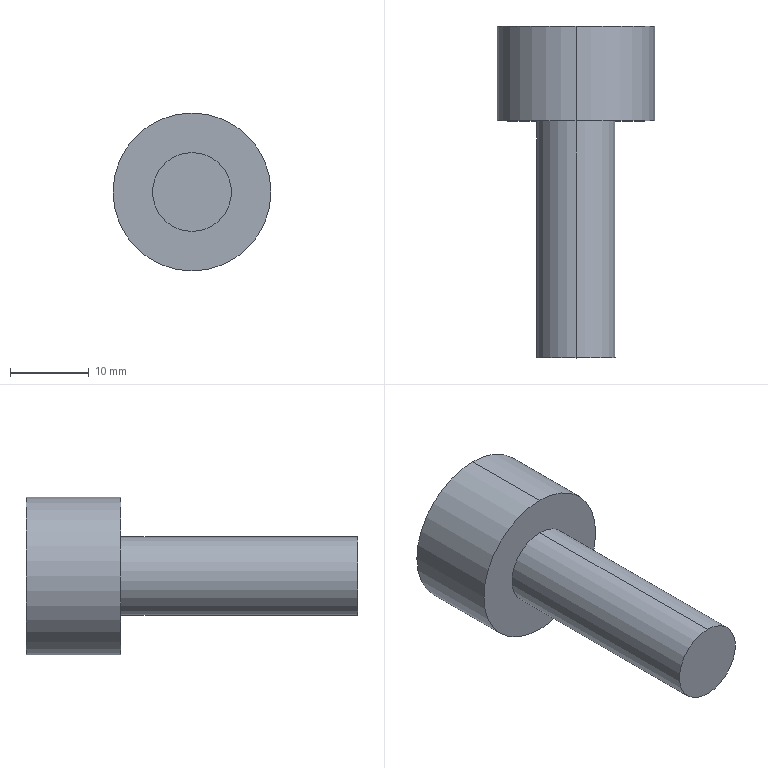Part | SolidWorks | features ICE 2, Extrusion 1 | 1 solid | 14 faces | box 20 x 42 x 20 mm | volume 5300 mm3 | plane 10 | cylinder 4 | commonest cylinder face diameters 10 x2 20 x2
STEP:
#1=CARTESIAN_POINT('',(0.,42.,10.));
#2=VERTEX_POINT('',#1);
#3=CARTESIAN_POINT('',(0.,42.,-10.));
#4=VERTEX_POINT('',#3);
#5=CARTESIAN_POINT('',(0.,42.,0.));
#6=DIRECTION('',(0.,1.,0.));
#7=DIRECTION('',(0.,0.,1.));
#8=AXIS2_PLACEMENT_3D('',#5,#6,#7);
#9=CIRCLE('',#8,10.);
#10=EDGE_CURVE('',#2,#4,#9,.T.);
#11=ORIENTED_EDGE('',*,*,#10,.F.);
#12=CARTESIAN_POINT('',(0.,30.,10.));
#13=VERTEX_POINT('',#12);
#14=CARTESIAN_POINT('',(0.,42.,10.));
#15=DIRECTION('',(0.,-1.,0.));
#16=VECTOR('',#15,1000.);
#17=LINE('',#14,#16);
#18=EDGE_CURVE('',#2,#13,#17,.T.);
#19=ORIENTED_EDGE('',*,*,#18,.T.);
#20=CARTESIAN_POINT('',(0.,30.,-10.));
#21=VERTEX_POINT('',#20);
#22=CARTESIAN_POINT('',(0.,30.,0.));
#23=DIRECTION('',(0.,1.,0.));
#24=DIRECTION('',(0.,0.,1.));
#25=AXIS2_PLACEMENT_3D('',#22,#23,#24);
#26=CIRCLE('',#25,10.);
#27=EDGE_CURVE('',#13,#21,#26,.T.);
#28=ORIENTED_EDGE('',*,*,#27,.T.);
#29=CARTESIAN_POINT('',(0.,42.,-10.));
#30=DIRECTION('',(0.,-1.,0.));
#31=VECTOR('',#30,1000.);
#32=LINE('',#29,#31);
#33=EDGE_CURVE('',#4,#21,#32,.T.);
#34=ORIENTED_EDGE('',*,*,#33,.F.);
#35=EDGE_LOOP('',(#11,#19,#28,#34));
#36=FACE_OUTER_BOUND('',#35,.T.);
#37=CARTESIAN_POINT('',(0.,42.,0.));
#38=DIRECTION('',(0.,-1.,0.));
#39=DIRECTION('',(0.,0.,-1.));
#40=AXIS2_PLACEMENT_3D('',#37,#38,#39);
#41=CYLINDRICAL_SURFACE('',#40,10.);
#42=ADVANCED_FACE('',(#36),#41,.T.);
#43=CARTESIAN_POINT('',(0.,30.,5.));
#44=VERTEX_POINT('',#43);
#45=CARTESIAN_POINT('',(0.,30.,-5.));
#46=VERTEX_POINT('',#45);
#47=CARTESIAN_POINT('',(0.,30.,0.));
#48=DIRECTION('',(0.,1.,0.));
#49=DIRECTION('',(0.,0.,1.));
#50=AXIS2_PLACEMENT_3D('',#47,#48,#49);
#51=CIRCLE('',#50,5.);
#52=EDGE_CURVE('',#44,#46,#51,.T.);
#53=ORIENTED_EDGE('',*,*,#52,.F.);
#54=CARTESIAN_POINT('',(0.,0.,5.));
#55=VERTEX_POINT('',#54);
#56=CARTESIAN_POINT('',(0.,30.,5.));
#57=DIRECTION('',(0.,-1.,0.));
#58=VECTOR('',#57,1000.);
#59=LINE('',#56,#58);
#60=EDGE_CURVE('',#44,#55,#59,.T.);
#61=ORIENTED_EDGE('',*,*,#60,.T.);
#62=CARTESIAN_POINT('',(0.,0.,-5.));
#63=VERTEX_POINT('',#62);
#64=CARTESIAN_POINT('',(0.,0.,0.));
#65=DIRECTION('',(0.,1.,0.));
#66=DIRECTION('',(0.,0.,1.));
#67=AXIS2_PLACEMENT_3D('',#64,#65,#66);
#68=CIRCLE('',#67,5.);
#69=EDGE_CURVE('',#55,#63,#68,.T.);
#70=ORIENTED_EDGE('',*,*,#69,.T.);
#71=CARTESIAN_POINT('',(0.,30.,-5.));
#72=DIRECTION('',(0.,-1.,0.));
#73=VECTOR('',#72,1000.);
#74=LINE('',#71,#73);
#75=EDGE_CURVE('',#46,#63,#74,.T.);
#76=ORIENTED_EDGE('',*,*,#75,.F.);
#77=EDGE_LOOP('',(#53,#61,#70,#76));
#78=FACE_OUTER_BOUND('',#77,.T.);
#79=CARTESIAN_POINT('',(0.,30.,0.));
#80=DIRECTION('',(0.,-1.,0.));
#81=DIRECTION('',(0.,0.,-1.));
#82=AXIS2_PLACEMENT_3D('',#79,#80,#81);
#83=CYLINDRICAL_SURFACE('',#82,5.);
#84=ADVANCED_FACE('',(#78),#83,.T.);
#85=ORIENTED_EDGE('',*,*,#60,.F.);
#86=CARTESIAN_POINT('',(0.,30.,0.));
#87=DIRECTION('',(0.,1.,0.));
#88=DIRECTION('',(0.,0.,1.));
#89=AXIS2_PLACEMENT_3D('',#86,#87,#88);
#90=CIRCLE('',#89,5.);
#91=EDGE_CURVE('',#46,#44,#90,.T.);
#92=ORIENTED_EDGE('',*,*,#91,.F.);
#93=ORIENTED_EDGE('',*,*,#75,.T.);
#94=CARTESIAN_POINT('',(0.,0.,0.));
#95=DIRECTION('',(0.,1.,0.));
#96=DIRECTION('',(0.,0.,1.));
#97=AXIS2_PLACEMENT_3D('',#94,#95,#96);
#98=CIRCLE('',#97,5.);
#99=EDGE_CURVE('',#63,#55,#98,.T.);
#100=ORIENTED_EDGE('',*,*,#99,.T.);
#101=EDGE_LOOP('',(#85,#92,#93,#100));
#102=FACE_OUTER_BOUND('',#101,.T.);
#103=CARTESIAN_POINT('',(0.,30.,0.));
#104=DIRECTION('',(0.,-1.,0.));
#105=DIRECTION('',(0.,0.,-1.));
#106=AXIS2_PLACEMENT_3D('',#103,#104,#105);
#107=CYLINDRICAL_SURFACE('',#106,5.);
#108=ADVANCED_FACE('',(#102),#107,.T.);
#109=ORIENTED_EDGE('',*,*,#99,.F.);
#110=ORIENTED_EDGE('',*,*,#69,.F.);
#111=EDGE_LOOP('',(#109,#110));
#112=FACE_OUTER_BOUND('',#111,.T.);
#113=CARTESIAN_POINT('',(0.,0.,0.));
#114=DIRECTION('',(0.,1.,0.));
#115=DIRECTION('',(0.,0.,1.));
#116=AXIS2_PLACEMENT_3D('',#113,#114,#115);
#117=PLANE('',#116);
#118=ADVANCED_FACE('',(#112),#117,.F.);
#119=ORIENTED_EDGE('',*,*,#18,.F.);
#120=CARTESIAN_POINT('',(0.,42.,0.));
#121=DIRECTION('',(0.,1.,0.));
#122=DIRECTION('',(0.,0.,1.));
#123=AXIS2_PLACEMENT_3D('',#120,#121,#122);
#124=CIRCLE('',#123,10.);
#125=EDGE_CURVE('',#4,#2,#124,.T.);
#126=ORIENTED_EDGE('',*,*,#125,.F.);
#127=ORIENTED_EDGE('',*,*,#33,.T.);
#128=CARTESIAN_POINT('',(0.,30.,0.));
#129=DIRECTION('',(0.,1.,0.));
#130=DIRECTION('',(0.,0.,1.));
#131=AXIS2_PLACEMENT_3D('',#128,#129,#130);
#132=CIRCLE('',#131,10.);
#133=EDGE_CURVE('',#21,#13,#132,.T.);
#134=ORIENTED_EDGE('',*,*,#133,.T.);
#135=EDGE_LOOP('',(#119,#126,#127,#134));
#136=FACE_OUTER_BOUND('',#135,.T.);
#137=CARTESIAN_POINT('',(0.,42.,0.));
#138=DIRECTION('',(0.,-1.,0.));
#139=DIRECTION('',(0.,0.,-1.));
#140=AXIS2_PLACEMENT_3D('',#137,#138,#139);
#141=CYLINDRICAL_SURFACE('',#140,10.);
#142=ADVANCED_FACE('',(#136),#141,.T.);
#143=CARTESIAN_POINT('',(-1.443,42.,6.138));
#144=VERTEX_POINT('',#143);
#145=CARTESIAN_POINT('',(4.594,42.,4.319));
#146=VERTEX_POINT('',#145);
#147=CARTESIAN_POINT('',(-1.443,42.,6.138));
#148=DIRECTION('',(0.9575,0.,-0.2885));
#149=VECTOR('',#148,1000.);
#150=LINE('',#147,#149);
#151=EDGE_CURVE('',#144,#146,#150,.T.);
#152=ORIENTED_EDGE('',*,*,#151,.F.);
#153=CARTESIAN_POINT('',(-6.037,42.,1.819));
#154=VERTEX_POINT('',#153);
#155=CARTESIAN_POINT('',(-6.037,42.,1.819));
#156=DIRECTION('',(0.7286,0.,0.6849));
#157=VECTOR('',#156,1000.);
#158=LINE('',#155,#157);
#159=EDGE_CURVE('',#154,#144,#158,.T.);
#160=ORIENTED_EDGE('',*,*,#159,.F.);
#161=CARTESIAN_POINT('',(-4.594,42.,-4.319));
#162=VERTEX_POINT('',#161);
#163=CARTESIAN_POINT('',(-4.594,42.,-4.319));
#164=DIRECTION('',(-0.2289,0.,0.9735));
#165=VECTOR('',#164,1000.);
#166=LINE('',#163,#165);
#167=EDGE_CURVE('',#162,#154,#166,.T.);
#168=ORIENTED_EDGE('',*,*,#167,.F.);
#169=CARTESIAN_POINT('',(1.443,42.,-6.138));
#170=VERTEX_POINT('',#169);
#171=CARTESIAN_POINT('',(1.443,42.,-6.138));
#172=DIRECTION('',(-0.9575,0.,0.2885));
#173=VECTOR('',#172,1000.);
#174=LINE('',#171,#173);
#175=EDGE_CURVE('',#170,#162,#174,.T.);
#176=ORIENTED_EDGE('',*,*,#175,.F.);
#177=CARTESIAN_POINT('',(6.037,42.,-1.819));
#178=VERTEX_POINT('',#177);
#179=CARTESIAN_POINT('',(6.037,42.,-1.819));
#180=DIRECTION('',(-0.7286,0.,-0.6849));
#181=VECTOR('',#180,1000.);
#182=LINE('',#179,#181);
#183=EDGE_CURVE('',#178,#170,#182,.T.);
#184=ORIENTED_EDGE('',*,*,#183,.F.);
#185=CARTESIAN_POINT('',(4.594,42.,4.319));
#186=DIRECTION('',(0.2289,0.,-0.9735));
#187=VECTOR('',#186,1000.);
#188=LINE('',#185,#187);
#189=EDGE_CURVE('',#146,#178,#188,.T.);
#190=ORIENTED_EDGE('',*,*,#189,.F.);
#191=EDGE_LOOP('',(#152,#160,#168,#176,#184,#190));
#192=FACE_BOUND('',#191,.T.);
#193=ORIENTED_EDGE('',*,*,#125,.T.);
#194=ORIENTED_EDGE('',*,*,#10,.T.);
#195=EDGE_LOOP('',(#193,#194));
#196=FACE_OUTER_BOUND('',#195,.T.);
#197=CARTESIAN_POINT('',(0.,42.,0.));
#198=DIRECTION('',(0.,1.,0.));
#199=DIRECTION('',(0.,0.,1.));
#200=AXIS2_PLACEMENT_3D('',#197,#198,#199);
#201=PLANE('',#200);
#202=ADVANCED_FACE('',(#192,#196),#201,.T.);
#203=ORIENTED_EDGE('',*,*,#91,.T.);
#204=ORIENTED_EDGE('',*,*,#52,.T.);
#205=EDGE_LOOP('',(#203,#204));
#206=FACE_BOUND('',#205,.T.);
#207=ORIENTED_EDGE('',*,*,#133,.F.);
#208=ORIENTED_EDGE('',*,*,#27,.F.);
#209=EDGE_LOOP('',(#207,#208));
#210=FACE_OUTER_BOUND('',#209,.T.);
#211=CARTESIAN_POINT('',(0.,30.,0.));
#212=DIRECTION('',(0.,1.,0.));
#213=DIRECTION('',(0.,0.,1.));
#214=AXIS2_PLACEMENT_3D('',#211,#212,#213);
#215=PLANE('',#214);
#216=ADVANCED_FACE('',(#206,#210),#215,.F.);
#217=ORIENTED_EDGE('',*,*,#151,.T.);
#218=CARTESIAN_POINT('',(4.594,34.,4.319));
#219=VERTEX_POINT('',#218);
#220=CARTESIAN_POINT('',(4.594,34.,4.319));
#221=DIRECTION('',(0.,1.,0.));
#222=VECTOR('',#221,1000.);
#223=LINE('',#220,#222);
#224=EDGE_CURVE('',#219,#146,#223,.T.);
#225=ORIENTED_EDGE('',*,*,#224,.F.);
#226=CARTESIAN_POINT('',(-1.443,34.,6.138));
#227=VERTEX_POINT('',#226);
#228=CARTESIAN_POINT('',(-1.443,34.,6.138));
#229=DIRECTION('',(0.9575,0.,-0.2885));
#230=VECTOR('',#229,1000.);
#231=LINE('',#228,#230);
#232=EDGE_CURVE('',#227,#219,#231,.T.);
#233=ORIENTED_EDGE('',*,*,#232,.F.);
#234=CARTESIAN_POINT('',(-1.443,34.,6.138));
#235=DIRECTION('',(0.,1.,0.));
#236=VECTOR('',#235,1000.);
#237=LINE('',#234,#236);
#238=EDGE_CURVE('',#227,#144,#237,.T.);
#239=ORIENTED_EDGE('',*,*,#238,.T.);
#240=EDGE_LOOP('',(#217,#225,#233,#239));
#241=FACE_OUTER_BOUND('',#240,.T.);
#242=CARTESIAN_POINT('',(-1.443,34.,6.138));
#243=DIRECTION('',(0.2885,0.,0.9575));
#244=DIRECTION('',(0.9575,0.,-0.2885));
#245=AXIS2_PLACEMENT_3D('',#242,#243,#244);
#246=PLANE('',#245);
#247=ADVANCED_FACE('',(#241),#246,.F.);
#248=ORIENTED_EDGE('',*,*,#159,.T.);
#249=ORIENTED_EDGE('',*,*,#238,.F.);
#250=CARTESIAN_POINT('',(-6.037,34.,1.819));
#251=VERTEX_POINT('',#250);
#252=CARTESIAN_POINT('',(-6.037,34.,1.819));
#253=DIRECTION('',(0.7286,0.,0.6849));
#254=VECTOR('',#253,1000.);
#255=LINE('',#252,#254);
#256=EDGE_CURVE('',#251,#227,#255,.T.);
#257=ORIENTED_EDGE('',*,*,#256,.F.);
#258=CARTESIAN_POINT('',(-6.037,34.,1.819));
#259=DIRECTION('',(0.,1.,0.));
#260=VECTOR('',#259,1000.);
#261=LINE('',#258,#260);
#262=EDGE_CURVE('',#251,#154,#261,.T.);
#263=ORIENTED_EDGE('',*,*,#262,.T.);
#264=EDGE_LOOP('',(#248,#249,#257,#263));
#265=FACE_OUTER_BOUND('',#264,.T.);
#266=CARTESIAN_POINT('',(-6.037,34.,1.819));
#267=DIRECTION('',(-0.6849,0.,0.7286));
#268=DIRECTION('',(0.7286,0.,0.6849));
#269=AXIS2_PLACEMENT_3D('',#266,#267,#268);
#270=PLANE('',#269);
#271=ADVANCED_FACE('',(#265),#270,.F.);
#272=ORIENTED_EDGE('',*,*,#167,.T.);
#273=ORIENTED_EDGE('',*,*,#262,.F.);
#274=CARTESIAN_POINT('',(-4.594,34.,-4.319));
#275=VERTEX_POINT('',#274);
#276=CARTESIAN_POINT('',(-4.594,34.,-4.319));
#277=DIRECTION('',(-0.2289,0.,0.9735));
#278=VECTOR('',#277,1000.);
#279=LINE('',#276,#278);
#280=EDGE_CURVE('',#275,#251,#279,.T.);
#281=ORIENTED_EDGE('',*,*,#280,.F.);
#282=CARTESIAN_POINT('',(-4.594,34.,-4.319));
#283=DIRECTION('',(0.,1.,0.));
#284=VECTOR('',#283,1000.);
#285=LINE('',#282,#284);
#286=EDGE_CURVE('',#275,#162,#285,.T.);
#287=ORIENTED_EDGE('',*,*,#286,.T.);
#288=EDGE_LOOP('',(#272,#273,#281,#287));
#289=FACE_OUTER_BOUND('',#288,.T.);
#290=CARTESIAN_POINT('',(-4.594,34.,-4.319));
#291=DIRECTION('',(-0.9735,0.,-0.2289));
#292=DIRECTION('',(-0.2289,0.,0.9735));
#293=AXIS2_PLACEMENT_3D('',#290,#291,#292);
#294=PLANE('',#293);
#295=ADVANCED_FACE('',(#289),#294,.F.);
#296=ORIENTED_EDGE('',*,*,#175,.T.);
#297=ORIENTED_EDGE('',*,*,#286,.F.);
#298=CARTESIAN_POINT('',(1.443,34.,-6.138));
#299=VERTEX_POINT('',#298);
#300=CARTESIAN_POINT('',(1.443,34.,-6.138));
#301=DIRECTION('',(-0.9575,0.,0.2885));
#302=VECTOR('',#301,1000.);
#303=LINE('',#300,#302);
#304=EDGE_CURVE('',#299,#275,#303,.T.);
#305=ORIENTED_EDGE('',*,*,#304,.F.);
#306=CARTESIAN_POINT('',(1.443,34.,-6.138));
#307=DIRECTION('',(0.,1.,0.));
#308=VECTOR('',#307,1000.);
#309=LINE('',#306,#308);
#310=EDGE_CURVE('',#299,#170,#309,.T.);
#311=ORIENTED_EDGE('',*,*,#310,.T.);
#312=EDGE_LOOP('',(#296,#297,#305,#311));
#313=FACE_OUTER_BOUND('',#312,.T.);
#314=CARTESIAN_POINT('',(1.443,34.,-6.138));
#315=DIRECTION('',(-0.2885,0.,-0.9575));
#316=DIRECTION('',(-0.9575,0.,0.2885));
#317=AXIS2_PLACEMENT_3D('',#314,#315,#316);
#318=PLANE('',#317);
#319=ADVANCED_FACE('',(#313),#318,.F.);
#320=ORIENTED_EDGE('',*,*,#183,.T.);
#321=ORIENTED_EDGE('',*,*,#310,.F.);
#322=CARTESIAN_POINT('',(6.037,34.,-1.819));
#323=VERTEX_POINT('',#322);
#324=CARTESIAN_POINT('',(6.037,34.,-1.819));
#325=DIRECTION('',(-0.7286,0.,-0.6849));
#326=VECTOR('',#325,1000.);
#327=LINE('',#324,#326);
#328=EDGE_CURVE('',#323,#299,#327,.T.);
#329=ORIENTED_EDGE('',*,*,#328,.F.);
#330=CARTESIAN_POINT('',(6.037,34.,-1.819));
#331=DIRECTION('',(0.,1.,0.));
#332=VECTOR('',#331,1000.);
#333=LINE('',#330,#332);
#334=EDGE_CURVE('',#323,#178,#333,.T.);
#335=ORIENTED_EDGE('',*,*,#334,.T.);
#336=EDGE_LOOP('',(#320,#321,#329,#335));
#337=FACE_OUTER_BOUND('',#336,.T.);
#338=CARTESIAN_POINT('',(6.037,34.,-1.819));
#339=DIRECTION('',(0.6849,0.,-0.7286));
#340=DIRECTION('',(-0.7286,0.,-0.6849));
#341=AXIS2_PLACEMENT_3D('',#338,#339,#340);
#342=PLANE('',#341);
#343=ADVANCED_FACE('',(#337),#342,.F.);
#344=ORIENTED_EDGE('',*,*,#189,.T.);
#345=ORIENTED_EDGE('',*,*,#334,.F.);
#346=CARTESIAN_POINT('',(4.594,34.,4.319));
#347=DIRECTION('',(0.2289,0.,-0.9735));
#348=VECTOR('',#347,1000.);
#349=LINE('',#346,#348);
#350=EDGE_CURVE('',#219,#323,#349,.T.);
#351=ORIENTED_EDGE('',*,*,#350,.F.);
#352=ORIENTED_EDGE('',*,*,#224,.T.);
#353=EDGE_LOOP('',(#344,#345,#351,#352));
#354=FACE_OUTER_BOUND('',#353,.T.);
#355=CARTESIAN_POINT('',(4.594,34.,4.319));
#356=DIRECTION('',(0.9735,0.,0.2289));
#357=DIRECTION('',(0.2289,0.,-0.9735));
#358=AXIS2_PLACEMENT_3D('',#355,#356,#357);
#359=PLANE('',#358);
#360=ADVANCED_FACE('',(#354),#359,.F.);
#361=ORIENTED_EDGE('',*,*,#232,.T.);
#362=ORIENTED_EDGE('',*,*,#350,.T.);
#363=ORIENTED_EDGE('',*,*,#328,.T.);
#364=ORIENTED_EDGE('',*,*,#304,.T.);
#365=ORIENTED_EDGE('',*,*,#280,.T.);
#366=ORIENTED_EDGE('',*,*,#256,.T.);
#367=EDGE_LOOP('',(#361,#362,#363,#364,#365,#366));
#368=FACE_OUTER_BOUND('',#367,.T.);
#369=CARTESIAN_POINT('',(0.,34.,0.));
#370=DIRECTION('',(0.,1.,0.));
#371=DIRECTION('',(0.,0.,1.));
#372=AXIS2_PLACEMENT_3D('',#369,#370,#371);
#373=PLANE('',#372);
#374=ADVANCED_FACE('',(#368),#373,.T.);
#375=CLOSED_SHELL('',(#42,#84,#108,#118,#142,#202,#216,#247,#271,#295,#319,#343,#360,#374));
#376=MANIFOLD_SOLID_BREP('',#375);
#377=CARTESIAN_POINT('',(0.,0.,0.));
#378=DIRECTION('',(0.,0.,1.));
#379=DIRECTION('',(1.,0.,0.));
#380=AXIS2_PLACEMENT_3D('',#377,#378,#379);
#381=(LENGTH_UNIT()NAMED_UNIT(*)SI_UNIT(.MILLI.,.METRE.));
#382=UNCERTAINTY_MEASURE_WITH_UNIT(LENGTH_MEASURE(0.00001),#381,'','');
#383=(NAMED_UNIT(*)PLANE_ANGLE_UNIT()SI_UNIT($,.RADIAN.));
#384=(NAMED_UNIT(*)SI_UNIT($,.STERADIAN.)SOLID_ANGLE_UNIT());
#385=(GEOMETRIC_REPRESENTATION_CONTEXT(3)GLOBAL_UNCERTAINTY_ASSIGNED_CONTEXT((#382))GLOBAL_UNIT_ASSIGNED_CONTEXT((#381,#383,#384))REPRESENTATION_CONTEXT('',''));
#386=ADVANCED_BREP_SHAPE_REPRESENTATION('',(#376,#380),#385);